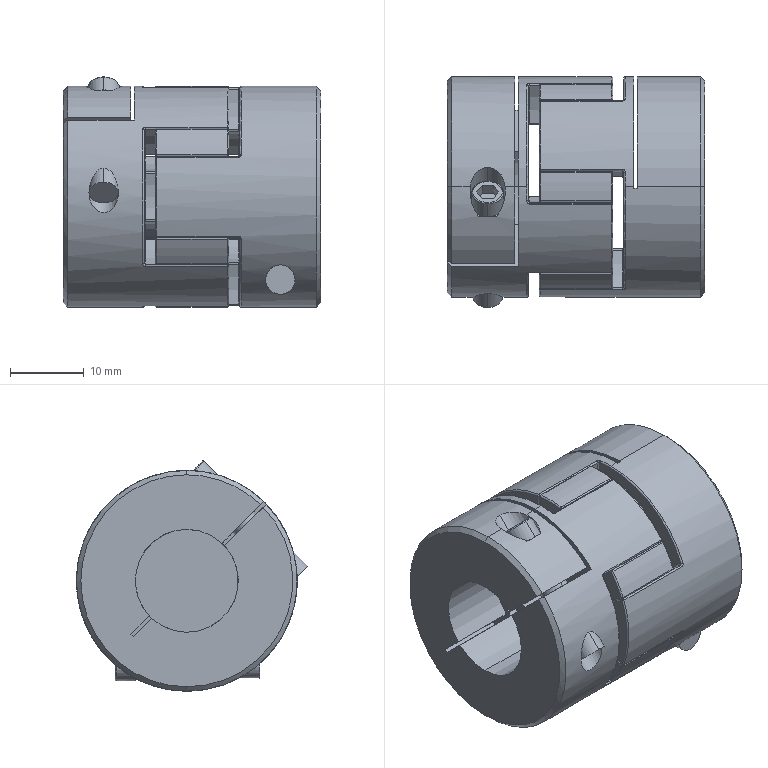Part | SolidWorks | features ICE 26, Fillet 5, CirPattern 4, Chamfer 2, Extrusion 2, Revolution 2 | 3 solids | 406 faces | box 35 x 31.403 x 31.299 mm | volume 17707 mm3 | torus 146 | cylinder 135 | sphere 58 | plane 50 | spline 12 | cone 5 | commonest cylinder face diameters 0.4 x58 18 x36 30 x13 4 x10 14 x4 14.4 x4